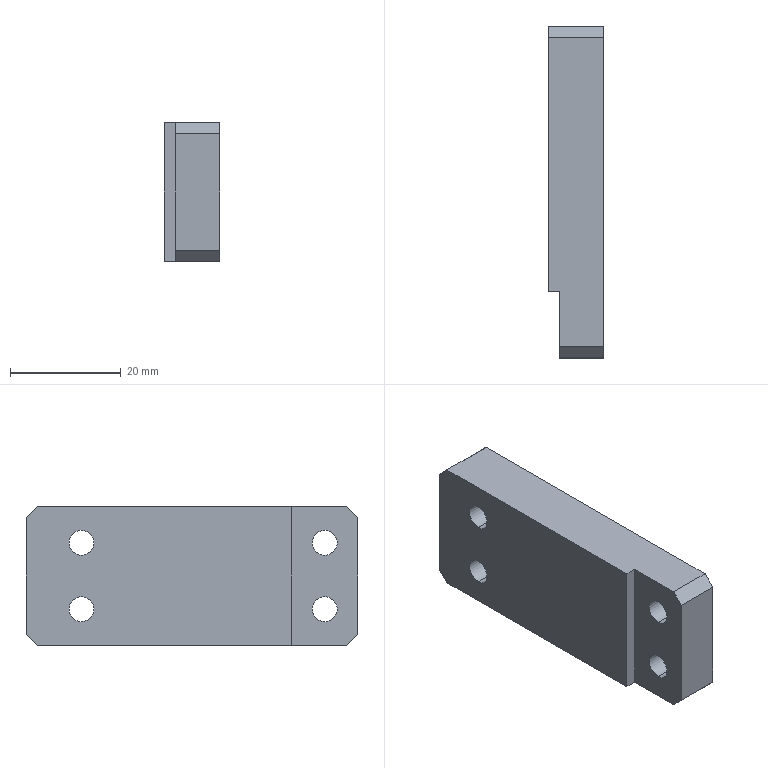Part | SolidWorks | features HoleWzd 2, Chamfer 1, Extrusion 1, ICE 1 | 1 solid | 32 faces | box 10 x 60 x 25 mm | volume 13123 mm3 | cylinder 16 | plane 16 | commonest cylinder face diameters 4.5 x8 8 x8
STEP:
#1=CARTESIAN_POINT('',(5.4,20.,10.));
#2=VERTEX_POINT('',#1);
#3=CARTESIAN_POINT('',(5.4,20.,2.));
#4=VERTEX_POINT('',#3);
#5=CARTESIAN_POINT('',(5.4,20.,6.));
#6=DIRECTION('',(1.,0.,0.));
#7=DIRECTION('',(0.,0.,-1.));
#8=AXIS2_PLACEMENT_3D('',#5,#6,#7);
#9=CIRCLE('',#8,4.);
#10=EDGE_CURVE('',#2,#4,#9,.T.);
#11=ORIENTED_EDGE('',*,*,#10,.F.);
#12=CARTESIAN_POINT('',(10.,20.,10.));
#13=VERTEX_POINT('',#12);
#14=CARTESIAN_POINT('',(10.,20.,10.));
#15=DIRECTION('',(1.,0.,0.));
#16=VECTOR('',#15,1000.);
#17=LINE('',#14,#16);
#18=EDGE_CURVE('',#2,#13,#17,.T.);
#19=ORIENTED_EDGE('',*,*,#18,.T.);
#20=CARTESIAN_POINT('',(10.,20.,2.));
#21=VERTEX_POINT('',#20);
#22=CARTESIAN_POINT('',(10.,20.,6.));
#23=DIRECTION('',(1.,0.,0.));
#24=DIRECTION('',(0.,0.,-1.));
#25=AXIS2_PLACEMENT_3D('',#22,#23,#24);
#26=CIRCLE('',#25,4.);
#27=EDGE_CURVE('',#13,#21,#26,.T.);
#28=ORIENTED_EDGE('',*,*,#27,.T.);
#29=CARTESIAN_POINT('',(10.,20.,2.));
#30=DIRECTION('',(1.,0.,0.));
#31=VECTOR('',#30,1000.);
#32=LINE('',#29,#31);
#33=EDGE_CURVE('',#4,#21,#32,.T.);
#34=ORIENTED_EDGE('',*,*,#33,.F.);
#35=EDGE_LOOP('',(#11,#19,#28,#34));
#36=FACE_OUTER_BOUND('',#35,.T.);
#37=CARTESIAN_POINT('',(10.,20.,6.));
#38=DIRECTION('',(1.,0.,0.));
#39=DIRECTION('',(0.,0.,-1.));
#40=AXIS2_PLACEMENT_3D('',#37,#38,#39);
#41=CYLINDRICAL_SURFACE('',#40,4.);
#42=ADVANCED_FACE('',(#36),#41,.F.);
#43=CARTESIAN_POINT('',(0.,20.,8.25));
#44=VERTEX_POINT('',#43);
#45=CARTESIAN_POINT('',(0.,20.,3.75));
#46=VERTEX_POINT('',#45);
#47=CARTESIAN_POINT('',(0.,20.,6.));
#48=DIRECTION('',(1.,0.,0.));
#49=DIRECTION('',(0.,0.,-1.));
#50=AXIS2_PLACEMENT_3D('',#47,#48,#49);
#51=CIRCLE('',#50,2.25);
#52=EDGE_CURVE('',#44,#46,#51,.T.);
#53=ORIENTED_EDGE('',*,*,#52,.F.);
#54=CARTESIAN_POINT('',(5.4,20.,8.25));
#55=VERTEX_POINT('',#54);
#56=CARTESIAN_POINT('',(10.,20.,8.25));
#57=DIRECTION('',(1.,0.,0.));
#58=VECTOR('',#57,1000.);
#59=LINE('',#56,#58);
#60=EDGE_CURVE('',#44,#55,#59,.T.);
#61=ORIENTED_EDGE('',*,*,#60,.T.);
#62=CARTESIAN_POINT('',(5.4,20.,3.75));
#63=VERTEX_POINT('',#62);
#64=CARTESIAN_POINT('',(5.4,20.,6.));
#65=DIRECTION('',(1.,0.,0.));
#66=DIRECTION('',(0.,0.,-1.));
#67=AXIS2_PLACEMENT_3D('',#64,#65,#66);
#68=CIRCLE('',#67,2.25);
#69=EDGE_CURVE('',#55,#63,#68,.T.);
#70=ORIENTED_EDGE('',*,*,#69,.T.);
#71=CARTESIAN_POINT('',(10.,20.,3.75));
#72=DIRECTION('',(1.,0.,0.));
#73=VECTOR('',#72,1000.);
#74=LINE('',#71,#73);
#75=EDGE_CURVE('',#46,#63,#74,.T.);
#76=ORIENTED_EDGE('',*,*,#75,.F.);
#77=EDGE_LOOP('',(#53,#61,#70,#76));
#78=FACE_OUTER_BOUND('',#77,.T.);
#79=CARTESIAN_POINT('',(10.,20.,6.));
#80=DIRECTION('',(1.,0.,0.));
#81=DIRECTION('',(0.,0.,-1.));
#82=AXIS2_PLACEMENT_3D('',#79,#80,#81);
#83=CYLINDRICAL_SURFACE('',#82,2.25);
#84=ADVANCED_FACE('',(#78),#83,.F.);
#85=CARTESIAN_POINT('',(5.4,20.,-2.));
#86=VERTEX_POINT('',#85);
#87=CARTESIAN_POINT('',(5.4,20.,-10.));
#88=VERTEX_POINT('',#87);
#89=CARTESIAN_POINT('',(5.4,20.,-6.));
#90=DIRECTION('',(1.,0.,0.));
#91=DIRECTION('',(0.,0.,-1.));
#92=AXIS2_PLACEMENT_3D('',#89,#90,#91);
#93=CIRCLE('',#92,4.);
#94=EDGE_CURVE('',#86,#88,#93,.T.);
#95=ORIENTED_EDGE('',*,*,#94,.F.);
#96=CARTESIAN_POINT('',(10.,20.,-2.));
#97=VERTEX_POINT('',#96);
#98=CARTESIAN_POINT('',(10.,20.,-2.));
#99=DIRECTION('',(1.,0.,0.));
#100=VECTOR('',#99,1000.);
#101=LINE('',#98,#100);
#102=EDGE_CURVE('',#86,#97,#101,.T.);
#103=ORIENTED_EDGE('',*,*,#102,.T.);
#104=CARTESIAN_POINT('',(10.,20.,-10.));
#105=VERTEX_POINT('',#104);
#106=CARTESIAN_POINT('',(10.,20.,-6.));
#107=DIRECTION('',(1.,0.,0.));
#108=DIRECTION('',(0.,0.,-1.));
#109=AXIS2_PLACEMENT_3D('',#106,#107,#108);
#110=CIRCLE('',#109,4.);
#111=EDGE_CURVE('',#97,#105,#110,.T.);
#112=ORIENTED_EDGE('',*,*,#111,.T.);
#113=CARTESIAN_POINT('',(10.,20.,-10.));
#114=DIRECTION('',(1.,0.,0.));
#115=VECTOR('',#114,1000.);
#116=LINE('',#113,#115);
#117=EDGE_CURVE('',#88,#105,#116,.T.);
#118=ORIENTED_EDGE('',*,*,#117,.F.);
#119=EDGE_LOOP('',(#95,#103,#112,#118));
#120=FACE_OUTER_BOUND('',#119,.T.);
#121=CARTESIAN_POINT('',(10.,20.,-6.));
#122=DIRECTION('',(1.,0.,0.));
#123=DIRECTION('',(0.,0.,-1.));
#124=AXIS2_PLACEMENT_3D('',#121,#122,#123);
#125=CYLINDRICAL_SURFACE('',#124,4.);
#126=ADVANCED_FACE('',(#120),#125,.F.);
#127=CARTESIAN_POINT('',(0.,20.,-3.75));
#128=VERTEX_POINT('',#127);
#129=CARTESIAN_POINT('',(0.,20.,-8.25));
#130=VERTEX_POINT('',#129);
#131=CARTESIAN_POINT('',(0.,20.,-6.));
#132=DIRECTION('',(1.,0.,0.));
#133=DIRECTION('',(0.,0.,-1.));
#134=AXIS2_PLACEMENT_3D('',#131,#132,#133);
#135=CIRCLE('',#134,2.25);
#136=EDGE_CURVE('',#128,#130,#135,.T.);
#137=ORIENTED_EDGE('',*,*,#136,.F.);
#138=CARTESIAN_POINT('',(5.4,20.,-3.75));
#139=VERTEX_POINT('',#138);
#140=CARTESIAN_POINT('',(10.,20.,-3.75));
#141=DIRECTION('',(1.,0.,0.));
#142=VECTOR('',#141,1000.);
#143=LINE('',#140,#142);
#144=EDGE_CURVE('',#128,#139,#143,.T.);
#145=ORIENTED_EDGE('',*,*,#144,.T.);
#146=CARTESIAN_POINT('',(5.4,20.,-8.25));
#147=VERTEX_POINT('',#146);
#148=CARTESIAN_POINT('',(5.4,20.,-6.));
#149=DIRECTION('',(1.,0.,0.));
#150=DIRECTION('',(0.,0.,-1.));
#151=AXIS2_PLACEMENT_3D('',#148,#149,#150);
#152=CIRCLE('',#151,2.25);
#153=EDGE_CURVE('',#139,#147,#152,.T.);
#154=ORIENTED_EDGE('',*,*,#153,.T.);
#155=CARTESIAN_POINT('',(10.,20.,-8.25));
#156=DIRECTION('',(1.,0.,0.));
#157=VECTOR('',#156,1000.);
#158=LINE('',#155,#157);
#159=EDGE_CURVE('',#130,#147,#158,.T.);
#160=ORIENTED_EDGE('',*,*,#159,.F.);
#161=EDGE_LOOP('',(#137,#145,#154,#160));
#162=FACE_OUTER_BOUND('',#161,.T.);
#163=CARTESIAN_POINT('',(10.,20.,-6.));
#164=DIRECTION('',(1.,0.,0.));
#165=DIRECTION('',(0.,0.,-1.));
#166=AXIS2_PLACEMENT_3D('',#163,#164,#165);
#167=CYLINDRICAL_SURFACE('',#166,2.25);
#168=ADVANCED_FACE('',(#162),#167,.F.);
#169=CARTESIAN_POINT('',(5.4,-24.,10.));
#170=VERTEX_POINT('',#169);
#171=CARTESIAN_POINT('',(5.4,-24.,2.));
#172=VERTEX_POINT('',#171);
#173=CARTESIAN_POINT('',(5.4,-24.,6.));
#174=DIRECTION('',(1.,0.,0.));
#175=DIRECTION('',(0.,0.,-1.));
#176=AXIS2_PLACEMENT_3D('',#173,#174,#175);
#177=CIRCLE('',#176,4.);
#178=EDGE_CURVE('',#170,#172,#177,.T.);
#179=ORIENTED_EDGE('',*,*,#178,.F.);
#180=CARTESIAN_POINT('',(10.,-24.,10.));
#181=VERTEX_POINT('',#180);
#182=CARTESIAN_POINT('',(10.,-24.,10.));
#183=DIRECTION('',(1.,0.,0.));
#184=VECTOR('',#183,1000.);
#185=LINE('',#182,#184);
#186=EDGE_CURVE('',#170,#181,#185,.T.);
#187=ORIENTED_EDGE('',*,*,#186,.T.);
#188=CARTESIAN_POINT('',(10.,-24.,2.));
#189=VERTEX_POINT('',#188);
#190=CARTESIAN_POINT('',(10.,-24.,6.));
#191=DIRECTION('',(1.,0.,0.));
#192=DIRECTION('',(0.,0.,-1.));
#193=AXIS2_PLACEMENT_3D('',#190,#191,#192);
#194=CIRCLE('',#193,4.);
#195=EDGE_CURVE('',#181,#189,#194,.T.);
#196=ORIENTED_EDGE('',*,*,#195,.T.);
#197=CARTESIAN_POINT('',(10.,-24.,2.));
#198=DIRECTION('',(1.,0.,0.));
#199=VECTOR('',#198,1000.);
#200=LINE('',#197,#199);
#201=EDGE_CURVE('',#172,#189,#200,.T.);
#202=ORIENTED_EDGE('',*,*,#201,.F.);
#203=EDGE_LOOP('',(#179,#187,#196,#202));
#204=FACE_OUTER_BOUND('',#203,.T.);
#205=CARTESIAN_POINT('',(10.,-24.,6.));
#206=DIRECTION('',(1.,0.,0.));
#207=DIRECTION('',(0.,0.,-1.));
#208=AXIS2_PLACEMENT_3D('',#205,#206,#207);
#209=CYLINDRICAL_SURFACE('',#208,4.);
#210=ADVANCED_FACE('',(#204),#209,.F.);
#211=CARTESIAN_POINT('',(2.,-24.,8.25));
#212=VERTEX_POINT('',#211);
#213=CARTESIAN_POINT('',(2.,-24.,3.75));
#214=VERTEX_POINT('',#213);
#215=CARTESIAN_POINT('',(2.,-24.,6.));
#216=DIRECTION('',(1.,0.,0.));
#217=DIRECTION('',(0.,0.,-1.));
#218=AXIS2_PLACEMENT_3D('',#215,#216,#217);
#219=CIRCLE('',#218,2.25);
#220=EDGE_CURVE('',#212,#214,#219,.T.);
#221=ORIENTED_EDGE('',*,*,#220,.F.);
#222=CARTESIAN_POINT('',(5.4,-24.,8.25));
#223=VERTEX_POINT('',#222);
#224=CARTESIAN_POINT('',(10.,-24.,8.25));
#225=DIRECTION('',(1.,0.,0.));
#226=VECTOR('',#225,1000.);
#227=LINE('',#224,#226);
#228=EDGE_CURVE('',#212,#223,#227,.T.);
#229=ORIENTED_EDGE('',*,*,#228,.T.);
#230=CARTESIAN_POINT('',(5.4,-24.,3.75));
#231=VERTEX_POINT('',#230);
#232=CARTESIAN_POINT('',(5.4,-24.,6.));
#233=DIRECTION('',(1.,0.,0.));
#234=DIRECTION('',(0.,0.,-1.));
#235=AXIS2_PLACEMENT_3D('',#232,#233,#234);
#236=CIRCLE('',#235,2.25);
#237=EDGE_CURVE('',#223,#231,#236,.T.);
#238=ORIENTED_EDGE('',*,*,#237,.T.);
#239=CARTESIAN_POINT('',(10.,-24.,3.75));
#240=DIRECTION('',(1.,0.,0.));
#241=VECTOR('',#240,1000.);
#242=LINE('',#239,#241);
#243=EDGE_CURVE('',#214,#231,#242,.T.);
#244=ORIENTED_EDGE('',*,*,#243,.F.);
#245=EDGE_LOOP('',(#221,#229,#238,#244));
#246=FACE_OUTER_BOUND('',#245,.T.);
#247=CARTESIAN_POINT('',(10.,-24.,6.));
#248=DIRECTION('',(1.,0.,0.));
#249=DIRECTION('',(0.,0.,-1.));
#250=AXIS2_PLACEMENT_3D('',#247,#248,#249);
#251=CYLINDRICAL_SURFACE('',#250,2.25);
#252=ADVANCED_FACE('',(#246),#251,.F.);
#253=CARTESIAN_POINT('',(5.4,-24.,-2.));
#254=VERTEX_POINT('',#253);
#255=CARTESIAN_POINT('',(5.4,-24.,-10.));
#256=VERTEX_POINT('',#255);
#257=CARTESIAN_POINT('',(5.4,-24.,-6.));
#258=DIRECTION('',(1.,0.,0.));
#259=DIRECTION('',(0.,0.,-1.));
#260=AXIS2_PLACEMENT_3D('',#257,#258,#259);
#261=CIRCLE('',#260,4.);
#262=EDGE_CURVE('',#254,#256,#261,.T.);
#263=ORIENTED_EDGE('',*,*,#262,.F.);
#264=CARTESIAN_POINT('',(10.,-24.,-2.));
#265=VERTEX_POINT('',#264);
#266=CARTESIAN_POINT('',(10.,-24.,-2.));
#267=DIRECTION('',(1.,0.,0.));
#268=VECTOR('',#267,1000.);
#269=LINE('',#266,#268);
#270=EDGE_CURVE('',#254,#265,#269,.T.);
#271=ORIENTED_EDGE('',*,*,#270,.T.);
#272=CARTESIAN_POINT('',(10.,-24.,-10.));
#273=VERTEX_POINT('',#272);
#274=CARTESIAN_POINT('',(10.,-24.,-6.));
#275=DIRECTION('',(1.,0.,0.));
#276=DIRECTION('',(0.,0.,-1.));
#277=AXIS2_PLACEMENT_3D('',#274,#275,#276);
#278=CIRCLE('',#277,4.);
#279=EDGE_CURVE('',#265,#273,#278,.T.);
#280=ORIENTED_EDGE('',*,*,#279,.T.);
#281=CARTESIAN_POINT('',(10.,-24.,-10.));
#282=DIRECTION('',(1.,0.,0.));
#283=VECTOR('',#282,1000.);
#284=LINE('',#281,#283);
#285=EDGE_CURVE('',#256,#273,#284,.T.);
#286=ORIENTED_EDGE('',*,*,#285,.F.);
#287=EDGE_LOOP('',(#263,#271,#280,#286));
#288=FACE_OUTER_BOUND('',#287,.T.);
#289=CARTESIAN_POINT('',(10.,-24.,-6.));
#290=DIRECTION('',(1.,0.,0.));
#291=DIRECTION('',(0.,0.,-1.));
#292=AXIS2_PLACEMENT_3D('',#289,#290,#291);
#293=CYLINDRICAL_SURFACE('',#292,4.);
#294=ADVANCED_FACE('',(#288),#293,.F.);
#295=CARTESIAN_POINT('',(2.,-24.,-3.75));
#296=VERTEX_POINT('',#295);
#297=CARTESIAN_POINT('',(2.,-24.,-8.25));
#298=VERTEX_POINT('',#297);
#299=CARTESIAN_POINT('',(2.,-24.,-6.));
#300=DIRECTION('',(1.,0.,0.));
#301=DIRECTION('',(0.,0.,-1.));
#302=AXIS2_PLACEMENT_3D('',#299,#300,#301);
#303=CIRCLE('',#302,2.25);
#304=EDGE_CURVE('',#296,#298,#303,.T.);
#305=ORIENTED_EDGE('',*,*,#304,.F.);
#306=CARTESIAN_POINT('',(5.4,-24.,-3.75));
#307=VERTEX_POINT('',#306);
#308=CARTESIAN_POINT('',(10.,-24.,-3.75));
#309=DIRECTION('',(1.,0.,0.));
#310=VECTOR('',#309,1000.);
#311=LINE('',#308,#310);
#312=EDGE_CURVE('',#296,#307,#311,.T.);
#313=ORIENTED_EDGE('',*,*,#312,.T.);
#314=CARTESIAN_POINT('',(5.4,-24.,-8.25));
#315=VERTEX_POINT('',#314);
#316=CARTESIAN_POINT('',(5.4,-24.,-6.));
#317=DIRECTION('',(1.,0.,0.));
#318=DIRECTION('',(0.,0.,-1.));
#319=AXIS2_PLACEMENT_3D('',#316,#317,#318);
#320=CIRCLE('',#319,2.25);
#321=EDGE_CURVE('',#307,#315,#320,.T.);
#322=ORIENTED_EDGE('',*,*,#321,.T.);
#323=CARTESIAN_POINT('',(10.,-24.,-8.25));
#324=DIRECTION('',(1.,0.,0.));
#325=VECTOR('',#324,1000.);
#326=LINE('',#323,#325);
#327=EDGE_CURVE('',#298,#315,#326,.T.);
#328=ORIENTED_EDGE('',*,*,#327,.F.);
#329=EDGE_LOOP('',(#305,#313,#322,#328));
#330=FACE_OUTER_BOUND('',#329,.T.);
#331=CARTESIAN_POINT('',(10.,-24.,-6.));
#332=DIRECTION('',(1.,0.,0.));
#333=DIRECTION('',(0.,0.,-1.));
#334=AXIS2_PLACEMENT_3D('',#331,#332,#333);
#335=CYLINDRICAL_SURFACE('',#334,2.25);
#336=ADVANCED_FACE('',(#330),#335,.F.);
#337=CARTESIAN_POINT('',(10.,20.,6.));
#338=DIRECTION('',(1.,0.,0.));
#339=DIRECTION('',(0.,0.,-1.));
#340=AXIS2_PLACEMENT_3D('',#337,#338,#339);
#341=CIRCLE('',#340,4.);
#342=EDGE_CURVE('',#21,#13,#341,.T.);
#343=ORIENTED_EDGE('',*,*,#342,.F.);
#344=ORIENTED_EDGE('',*,*,#27,.F.);
#345=EDGE_LOOP('',(#343,#344));
#346=FACE_BOUND('',#345,.T.);
#347=CARTESIAN_POINT('',(10.,20.,-6.));
#348=DIRECTION('',(1.,0.,0.));
#349=DIRECTION('',(0.,0.,-1.));
#350=AXIS2_PLACEMENT_3D('',#347,#348,#349);
#351=CIRCLE('',#350,4.);
#352=EDGE_CURVE('',#105,#97,#351,.T.);
#353=ORIENTED_EDGE('',*,*,#352,.F.);
#354=ORIENTED_EDGE('',*,*,#111,.F.);
#355=EDGE_LOOP('',(#353,#354));
#356=FACE_BOUND('',#355,.T.);
#357=CARTESIAN_POINT('',(10.,-24.,-6.));
#358=DIRECTION('',(1.,0.,0.));
#359=DIRECTION('',(0.,0.,-1.));
#360=AXIS2_PLACEMENT_3D('',#357,#358,#359);
#361=CIRCLE('',#360,4.);
#362=EDGE_CURVE('',#273,#265,#361,.T.);
#363=ORIENTED_EDGE('',*,*,#362,.F.);
#364=ORIENTED_EDGE('',*,*,#279,.F.);
#365=EDGE_LOOP('',(#363,#364));
#366=FACE_BOUND('',#365,.T.);
#367=CARTESIAN_POINT('',(10.,30.,-10.5));
#368=VERTEX_POINT('',#367);
#369=CARTESIAN_POINT('',(10.,30.,10.5));
#370=VERTEX_POINT('',#369);
#371=CARTESIAN_POINT('',(10.,30.,12.5));
#372=DIRECTION('',(0.,0.,1.));
#373=VECTOR('',#372,1000.);
#374=LINE('',#371,#373);
#375=EDGE_CURVE('',#368,#370,#374,.T.);
#376=ORIENTED_EDGE('',*,*,#375,.T.);
#377=CARTESIAN_POINT('',(10.,28.,12.5));
#378=VERTEX_POINT('',#377);
#379=CARTESIAN_POINT('',(10.,28.,12.5));
#380=DIRECTION('',(0.,-0.7071,0.7071));
#381=VECTOR('',#380,1000.);
#382=LINE('',#379,#381);
#383=EDGE_CURVE('',#370,#378,#382,.T.);
#384=ORIENTED_EDGE('',*,*,#383,.T.);
#385=CARTESIAN_POINT('',(10.,-28.,12.5));
#386=VERTEX_POINT('',#385);
#387=CARTESIAN_POINT('',(10.,-30.,12.5));
#388=DIRECTION('',(0.,-1.,0.));
#389=VECTOR('',#388,1000.);
#390=LINE('',#387,#389);
#391=EDGE_CURVE('',#378,#386,#390,.T.);
#392=ORIENTED_EDGE('',*,*,#391,.T.);
#393=CARTESIAN_POINT('',(10.,-30.,10.5));
#394=VERTEX_POINT('',#393);
#395=CARTESIAN_POINT('',(10.,-30.,10.5));
#396=DIRECTION('',(0.,-0.7071,-0.7071));
#397=VECTOR('',#396,1000.);
#398=LINE('',#395,#397);
#399=EDGE_CURVE('',#386,#394,#398,.T.);
#400=ORIENTED_EDGE('',*,*,#399,.T.);
#401=CARTESIAN_POINT('',(10.,-30.,-10.5));
#402=VERTEX_POINT('',#401);
#403=CARTESIAN_POINT('',(10.,-30.,12.5));
#404=DIRECTION('',(0.,0.,-1.));
#405=VECTOR('',#404,1000.);
#406=LINE('',#403,#405);
#407=EDGE_CURVE('',#394,#402,#406,.T.);
#408=ORIENTED_EDGE('',*,*,#407,.T.);
#409=CARTESIAN_POINT('',(10.,-28.,-12.5));
#410=VERTEX_POINT('',#409);
#411=CARTESIAN_POINT('',(10.,-28.,-12.5));
#412=DIRECTION('',(0.,0.7071,-0.7071));
#413=VECTOR('',#412,1000.);
#414=LINE('',#411,#413);
#415=EDGE_CURVE('',#402,#410,#414,.T.);
#416=ORIENTED_EDGE('',*,*,#415,.T.);
#417=CARTESIAN_POINT('',(10.,28.,-12.5));
#418=VERTEX_POINT('',#417);
#419=CARTESIAN_POINT('',(10.,-30.,-12.5));
#420=DIRECTION('',(0.,1.,0.));
#421=VECTOR('',#420,1000.);
#422=LINE('',#419,#421);
#423=EDGE_CURVE('',#410,#418,#422,.T.);
#424=ORIENTED_EDGE('',*,*,#423,.T.);
#425=CARTESIAN_POINT('',(10.,30.,-10.5));
#426=DIRECTION('',(0.,0.7071,0.7071));
#427=VECTOR('',#426,1000.);
#428=LINE('',#425,#427);
#429=EDGE_CURVE('',#418,#368,#428,.T.);
#430=ORIENTED_EDGE('',*,*,#429,.T.);
#431=EDGE_LOOP('',(#376,#384,#392,#400,#408,#416,#424,#430));
#432=FACE_OUTER_BOUND('',#431,.T.);
#433=CARTESIAN_POINT('',(10.,-24.,6.));
#434=DIRECTION('',(1.,0.,0.));
#435=DIRECTION('',(0.,0.,-1.));
#436=AXIS2_PLACEMENT_3D('',#433,#434,#435);
#437=CIRCLE('',#436,4.);
#438=EDGE_CURVE('',#189,#181,#437,.T.);
#439=ORIENTED_EDGE('',*,*,#438,.F.);
#440=ORIENTED_EDGE('',*,*,#195,.F.);
#441=EDGE_LOOP('',(#439,#440));
#442=FACE_BOUND('',#441,.T.);
#443=CARTESIAN_POINT('',(10.,0.,0.));
#444=DIRECTION('',(-1.,0.,0.));
#445=DIRECTION('',(0.,0.,1.));
#446=AXIS2_PLACEMENT_3D('',#443,#444,#445);
#447=PLANE('',#446);
#448=ADVANCED_FACE('',(#346,#356,#366,#432,#442),#447,.F.);
#449=CARTESIAN_POINT('',(0.,-18.,-12.5));
#450=VERTEX_POINT('',#449);
#451=CARTESIAN_POINT('',(0.,28.,-12.5));
#452=VERTEX_POINT('',#451);
#453=CARTESIAN_POINT('',(0.,-30.,-12.5));
#454=DIRECTION('',(0.,1.,0.));
#455=VECTOR('',#454,1000.);
#456=LINE('',#453,#455);
#457=EDGE_CURVE('',#450,#452,#456,.T.);
#458=ORIENTED_EDGE('',*,*,#457,.T.);
#459=CARTESIAN_POINT('',(10.,28.,-12.5));
#460=DIRECTION('',(1.,0.,0.));
#461=VECTOR('',#460,1000.);
#462=LINE('',#459,#461);
#463=EDGE_CURVE('',#452,#418,#462,.T.);
#464=ORIENTED_EDGE('',*,*,#463,.T.);
#465=ORIENTED_EDGE('',*,*,#423,.F.);
#466=CARTESIAN_POINT('',(2.,-28.,-12.5));
#467=VERTEX_POINT('',#466);
#468=CARTESIAN_POINT('',(10.,-28.,-12.5));
#469=DIRECTION('',(-1.,0.,0.));
#470=VECTOR('',#469,1000.);
#471=LINE('',#468,#470);
#472=EDGE_CURVE('',#410,#467,#471,.T.);
#473=ORIENTED_EDGE('',*,*,#472,.T.);
#474=CARTESIAN_POINT('',(2.,-18.,-12.5));
#475=VERTEX_POINT('',#474);
#476=CARTESIAN_POINT('',(2.,-30.,-12.5));
#477=DIRECTION('',(0.,-1.,0.));
#478=VECTOR('',#477,1000.);
#479=LINE('',#476,#478);
#480=EDGE_CURVE('',#475,#467,#479,.T.);
#481=ORIENTED_EDGE('',*,*,#480,.F.);
#482=CARTESIAN_POINT('',(2.,-18.,-12.5));
#483=DIRECTION('',(-1.,0.,0.));
#484=VECTOR('',#483,1000.);
#485=LINE('',#482,#484);
#486=EDGE_CURVE('',#475,#450,#485,.T.);
#487=ORIENTED_EDGE('',*,*,#486,.T.);
#488=EDGE_LOOP('',(#458,#464,#465,#473,#481,#487));
#489=FACE_OUTER_BOUND('',#488,.T.);
#490=CARTESIAN_POINT('',(10.,-30.,-12.5));
#491=DIRECTION('',(0.,0.,1.));
#492=DIRECTION('',(1.,0.,0.));
#493=AXIS2_PLACEMENT_3D('',#490,#491,#492);
#494=PLANE('',#493);
#495=ADVANCED_FACE('',(#489),#494,.F.);
#496=CARTESIAN_POINT('',(0.,30.,-10.5));
#497=VERTEX_POINT('',#496);
#498=CARTESIAN_POINT('',(0.,30.,10.5));
#499=VERTEX_POINT('',#498);
#500=CARTESIAN_POINT('',(0.,30.,12.5));
#501=DIRECTION('',(0.,0.,1.));
#502=VECTOR('',#501,1000.);
#503=LINE('',#500,#502);
#504=EDGE_CURVE('',#497,#499,#503,.T.);
#505=ORIENTED_EDGE('',*,*,#504,.T.);
#506=CARTESIAN_POINT('',(10.,30.,10.5));
#507=DIRECTION('',(1.,0.,0.));
#508=VECTOR('',#507,1000.);
#509=LINE('',#506,#508);
#510=EDGE_CURVE('',#499,#370,#509,.T.);
#511=ORIENTED_EDGE('',*,*,#510,.T.);
#512=ORIENTED_EDGE('',*,*,#375,.F.);
#513=CARTESIAN_POINT('',(10.,30.,-10.5));
#514=DIRECTION('',(-1.,0.,0.));
#515=VECTOR('',#514,1000.);
#516=LINE('',#513,#515);
#517=EDGE_CURVE('',#368,#497,#516,.T.);
#518=ORIENTED_EDGE('',*,*,#517,.T.);
#519=EDGE_LOOP('',(#505,#511,#512,#518));
#520=FACE_OUTER_BOUND('',#519,.T.);
#521=CARTESIAN_POINT('',(10.,30.,12.5));
#522=DIRECTION('',(0.,-1.,0.));
#523=DIRECTION('',(0.,0.,-1.));
#524=AXIS2_PLACEMENT_3D('',#521,#522,#523);
#525=PLANE('',#524);
#526=ADVANCED_FACE('',(#520),#525,.F.);
#527=ORIENTED_EDGE('',*,*,#391,.F.);
#528=CARTESIAN_POINT('',(0.,28.,12.5));
#529=VERTEX_POINT('',#528);
#530=CARTESIAN_POINT('',(10.,28.,12.5));
#531=DIRECTION('',(-1.,0.,0.));
#532=VECTOR('',#531,1000.);
#533=LINE('',#530,#532);
#534=EDGE_CURVE('',#378,#529,#533,.T.);
#535=ORIENTED_EDGE('',*,*,#534,.T.);
#536=CARTESIAN_POINT('',(0.,-18.,12.5));
#537=VERTEX_POINT('',#536);
#538=CARTESIAN_POINT('',(0.,-30.,12.5));
#539=DIRECTION('',(0.,-1.,0.));
#540=VECTOR('',#539,1000.);
#541=LINE('',#538,#540);
#542=EDGE_CURVE('',#529,#537,#541,.T.);
#543=ORIENTED_EDGE('',*,*,#542,.T.);
#544=CARTESIAN_POINT('',(2.,-18.,12.5));
#545=VERTEX_POINT('',#544);
#546=CARTESIAN_POINT('',(2.,-18.,12.5));
#547=DIRECTION('',(-1.,0.,0.));
#548=VECTOR('',#547,1000.);
#549=LINE('',#546,#548);
#550=EDGE_CURVE('',#545,#537,#549,.T.);
#551=ORIENTED_EDGE('',*,*,#550,.F.);
#552=CARTESIAN_POINT('',(2.,-28.,12.5));
#553=VERTEX_POINT('',#552);
#554=CARTESIAN_POINT('',(2.,-30.,12.5));
#555=DIRECTION('',(0.,1.,0.));
#556=VECTOR('',#555,1000.);
#557=LINE('',#554,#556);
#558=EDGE_CURVE('',#553,#545,#557,.T.);
#559=ORIENTED_EDGE('',*,*,#558,.F.);
#560=CARTESIAN_POINT('',(10.,-28.,12.5));
#561=DIRECTION('',(1.,0.,0.));
#562=VECTOR('',#561,1000.);
#563=LINE('',#560,#562);
#564=EDGE_CURVE('',#553,#386,#563,.T.);
#565=ORIENTED_EDGE('',*,*,#564,.T.);
#566=EDGE_LOOP('',(#527,#535,#543,#551,#559,#565));
#567=FACE_OUTER_BOUND('',#566,.T.);
#568=CARTESIAN_POINT('',(10.,-30.,12.5));
#569=DIRECTION('',(0.,0.,-1.));
#570=DIRECTION('',(-1.,0.,0.));
#571=AXIS2_PLACEMENT_3D('',#568,#569,#570);
#572=PLANE('',#571);
#573=ADVANCED_FACE('',(#567),#572,.F.);
#574=ORIENTED_EDGE('',*,*,#407,.F.);
#575=CARTESIAN_POINT('',(2.,-30.,10.5));
#576=VERTEX_POINT('',#575);
#577=CARTESIAN_POINT('',(10.,-30.,10.5));
#578=DIRECTION('',(-1.,0.,0.));
#579=VECTOR('',#578,1000.);
#580=LINE('',#577,#579);
#581=EDGE_CURVE('',#394,#576,#580,.T.);
#582=ORIENTED_EDGE('',*,*,#581,.T.);
#583=CARTESIAN_POINT('',(2.,-30.,-10.5));
#584=VERTEX_POINT('',#583);
#585=CARTESIAN_POINT('',(2.,-30.,-12.5));
#586=DIRECTION('',(0.,0.,1.));
#587=VECTOR('',#586,1000.);
#588=LINE('',#585,#587);
#589=EDGE_CURVE('',#584,#576,#588,.T.);
#590=ORIENTED_EDGE('',*,*,#589,.F.);
#591=CARTESIAN_POINT('',(10.,-30.,-10.5));
#592=DIRECTION('',(1.,0.,0.));
#593=VECTOR('',#592,1000.);
#594=LINE('',#591,#593);
#595=EDGE_CURVE('',#584,#402,#594,.T.);
#596=ORIENTED_EDGE('',*,*,#595,.T.);
#597=EDGE_LOOP('',(#574,#582,#590,#596));
#598=FACE_OUTER_BOUND('',#597,.T.);
#599=CARTESIAN_POINT('',(10.,-30.,12.5));
#600=DIRECTION('',(0.,1.,0.));
#601=DIRECTION('',(0.,0.,1.));
#602=AXIS2_PLACEMENT_3D('',#599,#600,#601);
#603=PLANE('',#602);
#604=ADVANCED_FACE('',(#598),#603,.F.);
#605=CARTESIAN_POINT('',(0.,20.,6.));
#606=DIRECTION('',(1.,0.,0.));
#607=DIRECTION('',(0.,0.,-1.));
#608=AXIS2_PLACEMENT_3D('',#605,#606,#607);
#609=CIRCLE('',#608,2.25);
#610=EDGE_CURVE('',#46,#44,#609,.T.);
#611=ORIENTED_EDGE('',*,*,#610,.T.);
#612=ORIENTED_EDGE('',*,*,#52,.T.);
#613=EDGE_LOOP('',(#611,#612));
#614=FACE_BOUND('',#613,.T.);
#615=CARTESIAN_POINT('',(0.,20.,-6.));
#616=DIRECTION('',(1.,0.,0.));
#617=DIRECTION('',(0.,0.,-1.));
#618=AXIS2_PLACEMENT_3D('',#615,#616,#617);
#619=CIRCLE('',#618,2.25);
#620=EDGE_CURVE('',#130,#128,#619,.T.);
#621=ORIENTED_EDGE('',*,*,#620,.T.);
#622=ORIENTED_EDGE('',*,*,#136,.T.);
#623=EDGE_LOOP('',(#621,#622));
#624=FACE_BOUND('',#623,.T.);
#625=ORIENTED_EDGE('',*,*,#542,.F.);
#626=CARTESIAN_POINT('',(0.,20.25,20.25));
#627=DIRECTION('',(0.,0.7071,-0.7071));
#628=VECTOR('',#627,1000.);
#629=LINE('',#626,#628);
#630=EDGE_CURVE('',#529,#499,#629,.T.);
#631=ORIENTED_EDGE('',*,*,#630,.T.);
#632=ORIENTED_EDGE('',*,*,#504,.F.);
#633=CARTESIAN_POINT('',(0.,20.25,-20.25));
#634=DIRECTION('',(0.,-0.7071,-0.7071));
#635=VECTOR('',#634,1000.);
#636=LINE('',#633,#635);
#637=EDGE_CURVE('',#497,#452,#636,.T.);
#638=ORIENTED_EDGE('',*,*,#637,.T.);
#639=ORIENTED_EDGE('',*,*,#457,.F.);
#640=CARTESIAN_POINT('',(0.,-18.,-12.5));
#641=DIRECTION('',(0.,0.,-1.));
#642=VECTOR('',#641,1000.);
#643=LINE('',#640,#642);
#644=EDGE_CURVE('',#537,#450,#643,.T.);
#645=ORIENTED_EDGE('',*,*,#644,.F.);
#646=EDGE_LOOP('',(#625,#631,#632,#638,#639,#645));
#647=FACE_OUTER_BOUND('',#646,.T.);
#648=CARTESIAN_POINT('',(0.,0.,0.));
#649=DIRECTION('',(-1.,0.,0.));
#650=DIRECTION('',(0.,0.,1.));
#651=AXIS2_PLACEMENT_3D('',#648,#649,#650);
#652=PLANE('',#651);
#653=ADVANCED_FACE('',(#614,#624,#647),#652,.T.);
#654=ORIENTED_EDGE('',*,*,#644,.T.);
#655=ORIENTED_EDGE('',*,*,#486,.F.);
#656=CARTESIAN_POINT('',(2.,-18.,-12.5));
#657=DIRECTION('',(0.,0.,-1.));
#658=VECTOR('',#657,1000.);
#659=LINE('',#656,#658);
#660=EDGE_CURVE('',#545,#475,#659,.T.);
#661=ORIENTED_EDGE('',*,*,#660,.F.);
#662=ORIENTED_EDGE('',*,*,#550,.T.);
#663=EDGE_LOOP('',(#654,#655,#661,#662));
#664=FACE_OUTER_BOUND('',#663,.T.);
#665=CARTESIAN_POINT('',(2.,-18.,-12.5));
#666=DIRECTION('',(0.,1.,0.));
#667=DIRECTION('',(0.,0.,1.));
#668=AXIS2_PLACEMENT_3D('',#665,#666,#667);
#669=PLANE('',#668);
#670=ADVANCED_FACE('',(#664),#669,.F.);
#671=CARTESIAN_POINT('',(2.,-24.,6.));
#672=DIRECTION('',(1.,0.,0.));
#673=DIRECTION('',(0.,0.,-1.));
#674=AXIS2_PLACEMENT_3D('',#671,#672,#673);
#675=CIRCLE('',#674,2.25);
#676=EDGE_CURVE('',#214,#212,#675,.T.);
#677=ORIENTED_EDGE('',*,*,#676,.T.);
#678=ORIENTED_EDGE('',*,*,#220,.T.);
#679=EDGE_LOOP('',(#677,#678));
#680=FACE_BOUND('',#679,.T.);
#681=CARTESIAN_POINT('',(2.,-24.,-6.));
#682=DIRECTION('',(1.,0.,0.));
#683=DIRECTION('',(0.,0.,-1.));
#684=AXIS2_PLACEMENT_3D('',#681,#682,#683);
#685=CIRCLE('',#684,2.25);
#686=EDGE_CURVE('',#298,#296,#685,.T.);
#687=ORIENTED_EDGE('',*,*,#686,.T.);
#688=ORIENTED_EDGE('',*,*,#304,.T.);
#689=EDGE_LOOP('',(#687,#688));
#690=FACE_BOUND('',#689,.T.);
#691=ORIENTED_EDGE('',*,*,#589,.T.);
#692=CARTESIAN_POINT('',(2.,-30.,10.5));
#693=DIRECTION('',(0.,0.7071,0.7071));
#694=VECTOR('',#693,1000.);
#695=LINE('',#692,#694);
#696=EDGE_CURVE('',#576,#553,#695,.T.);
#697=ORIENTED_EDGE('',*,*,#696,.T.);
#698=ORIENTED_EDGE('',*,*,#558,.T.);
#699=ORIENTED_EDGE('',*,*,#660,.T.);
#700=ORIENTED_EDGE('',*,*,#480,.T.);
#701=CARTESIAN_POINT('',(2.,-28.,-12.5));
#702=DIRECTION('',(0.,-0.7071,0.7071));
#703=VECTOR('',#702,1000.);
#704=LINE('',#701,#703);
#705=EDGE_CURVE('',#467,#584,#704,.T.);
#706=ORIENTED_EDGE('',*,*,#705,.T.);
#707=EDGE_LOOP('',(#691,#697,#698,#699,#700,#706));
#708=FACE_OUTER_BOUND('',#707,.T.);
#709=CARTESIAN_POINT('',(2.,0.,0.));
#710=DIRECTION('',(1.,0.,0.));
#711=DIRECTION('',(0.,0.,-1.));
#712=AXIS2_PLACEMENT_3D('',#709,#710,#711);
#713=PLANE('',#712);
#714=ADVANCED_FACE('',(#680,#690,#708),#713,.F.);
#715=ORIENTED_EDGE('',*,*,#312,.F.);
#716=ORIENTED_EDGE('',*,*,#686,.F.);
#717=ORIENTED_EDGE('',*,*,#327,.T.);
#718=CARTESIAN_POINT('',(5.4,-24.,-6.));
#719=DIRECTION('',(1.,0.,0.));
#720=DIRECTION('',(0.,0.,-1.));
#721=AXIS2_PLACEMENT_3D('',#718,#719,#720);
#722=CIRCLE('',#721,2.25);
#723=EDGE_CURVE('',#315,#307,#722,.T.);
#724=ORIENTED_EDGE('',*,*,#723,.T.);
#725=EDGE_LOOP('',(#715,#716,#717,#724));
#726=FACE_OUTER_BOUND('',#725,.T.);
#727=CARTESIAN_POINT('',(10.,-24.,-6.));
#728=DIRECTION('',(1.,0.,0.));
#729=DIRECTION('',(0.,0.,-1.));
#730=AXIS2_PLACEMENT_3D('',#727,#728,#729);
#731=CYLINDRICAL_SURFACE('',#730,2.25);
#732=ADVANCED_FACE('',(#726),#731,.F.);
#733=ORIENTED_EDGE('',*,*,#723,.F.);
#734=ORIENTED_EDGE('',*,*,#321,.F.);
#735=EDGE_LOOP('',(#733,#734));
#736=FACE_BOUND('',#735,.T.);
#737=CARTESIAN_POINT('',(5.4,-24.,-6.));
#738=DIRECTION('',(1.,0.,0.));
#739=DIRECTION('',(0.,0.,-1.));
#740=AXIS2_PLACEMENT_3D('',#737,#738,#739);
#741=CIRCLE('',#740,4.);
#742=EDGE_CURVE('',#256,#254,#741,.T.);
#743=ORIENTED_EDGE('',*,*,#742,.T.);
#744=ORIENTED_EDGE('',*,*,#262,.T.);
#745=EDGE_LOOP('',(#743,#744));
#746=FACE_OUTER_BOUND('',#745,.T.);
#747=CARTESIAN_POINT('',(5.4,-21.75,-6.));
#748=DIRECTION('',(-1.,0.,0.));
#749=DIRECTION('',(0.,0.,1.));
#750=AXIS2_PLACEMENT_3D('',#747,#748,#749);
#751=PLANE('',#750);
#752=ADVANCED_FACE('',(#736,#746),#751,.F.);
#753=ORIENTED_EDGE('',*,*,#270,.F.);
#754=ORIENTED_EDGE('',*,*,#742,.F.);
#755=ORIENTED_EDGE('',*,*,#285,.T.);
#756=ORIENTED_EDGE('',*,*,#362,.T.);
#757=EDGE_LOOP('',(#753,#754,#755,#756));
#758=FACE_OUTER_BOUND('',#757,.T.);
#759=CARTESIAN_POINT('',(10.,-24.,-6.));
#760=DIRECTION('',(1.,0.,0.));
#761=DIRECTION('',(0.,0.,-1.));
#762=AXIS2_PLACEMENT_3D('',#759,#760,#761);
#763=CYLINDRICAL_SURFACE('',#762,4.);
#764=ADVANCED_FACE('',(#758),#763,.F.);
#765=ORIENTED_EDGE('',*,*,#228,.F.);
#766=ORIENTED_EDGE('',*,*,#676,.F.);
#767=ORIENTED_EDGE('',*,*,#243,.T.);
#768=CARTESIAN_POINT('',(5.4,-24.,6.));
#769=DIRECTION('',(1.,0.,0.));
#770=DIRECTION('',(0.,0.,-1.));
#771=AXIS2_PLACEMENT_3D('',#768,#769,#770);
#772=CIRCLE('',#771,2.25);
#773=EDGE_CURVE('',#231,#223,#772,.T.);
#774=ORIENTED_EDGE('',*,*,#773,.T.);
#775=EDGE_LOOP('',(#765,#766,#767,#774));
#776=FACE_OUTER_BOUND('',#775,.T.);
#777=CARTESIAN_POINT('',(10.,-24.,6.));
#778=DIRECTION('',(1.,0.,0.));
#779=DIRECTION('',(0.,0.,-1.));
#780=AXIS2_PLACEMENT_3D('',#777,#778,#779);
#781=CYLINDRICAL_SURFACE('',#780,2.25);
#782=ADVANCED_FACE('',(#776),#781,.F.);
#783=ORIENTED_EDGE('',*,*,#773,.F.);
#784=ORIENTED_EDGE('',*,*,#237,.F.);
#785=EDGE_LOOP('',(#783,#784));
#786=FACE_BOUND('',#785,.T.);
#787=CARTESIAN_POINT('',(5.4,-24.,6.));
#788=DIRECTION('',(1.,0.,0.));
#789=DIRECTION('',(0.,0.,-1.));
#790=AXIS2_PLACEMENT_3D('',#787,#788,#789);
#791=CIRCLE('',#790,4.);
#792=EDGE_CURVE('',#172,#170,#791,.T.);
#793=ORIENTED_EDGE('',*,*,#792,.T.);
#794=ORIENTED_EDGE('',*,*,#178,.T.);
#795=EDGE_LOOP('',(#793,#794));
#796=FACE_OUTER_BOUND('',#795,.T.);
#797=CARTESIAN_POINT('',(5.4,-21.75,6.));
#798=DIRECTION('',(-1.,0.,0.));
#799=DIRECTION('',(0.,0.,1.));
#800=AXIS2_PLACEMENT_3D('',#797,#798,#799);
#801=PLANE('',#800);
#802=ADVANCED_FACE('',(#786,#796),#801,.F.);
#803=ORIENTED_EDGE('',*,*,#186,.F.);
#804=ORIENTED_EDGE('',*,*,#792,.F.);
#805=ORIENTED_EDGE('',*,*,#201,.T.);
#806=ORIENTED_EDGE('',*,*,#438,.T.);
#807=EDGE_LOOP('',(#803,#804,#805,#806));
#808=FACE_OUTER_BOUND('',#807,.T.);
#809=CARTESIAN_POINT('',(10.,-24.,6.));
#810=DIRECTION('',(1.,0.,0.));
#811=DIRECTION('',(0.,0.,-1.));
#812=AXIS2_PLACEMENT_3D('',#809,#810,#811);
#813=CYLINDRICAL_SURFACE('',#812,4.);
#814=ADVANCED_FACE('',(#808),#813,.F.);
#815=ORIENTED_EDGE('',*,*,#144,.F.);
#816=ORIENTED_EDGE('',*,*,#620,.F.);
#817=ORIENTED_EDGE('',*,*,#159,.T.);
#818=CARTESIAN_POINT('',(5.4,20.,-6.));
#819=DIRECTION('',(1.,0.,0.));
#820=DIRECTION('',(0.,0.,-1.));
#821=AXIS2_PLACEMENT_3D('',#818,#819,#820);
#822=CIRCLE('',#821,2.25);
#823=EDGE_CURVE('',#147,#139,#822,.T.);
#824=ORIENTED_EDGE('',*,*,#823,.T.);
#825=EDGE_LOOP('',(#815,#816,#817,#824));
#826=FACE_OUTER_BOUND('',#825,.T.);
#827=CARTESIAN_POINT('',(10.,20.,-6.));
#828=DIRECTION('',(1.,0.,0.));
#829=DIRECTION('',(0.,0.,-1.));
#830=AXIS2_PLACEMENT_3D('',#827,#828,#829);
#831=CYLINDRICAL_SURFACE('',#830,2.25);
#832=ADVANCED_FACE('',(#826),#831,.F.);
#833=ORIENTED_EDGE('',*,*,#823,.F.);
#834=ORIENTED_EDGE('',*,*,#153,.F.);
#835=EDGE_LOOP('',(#833,#834));
#836=FACE_BOUND('',#835,.T.);
#837=CARTESIAN_POINT('',(5.4,20.,-6.));
#838=DIRECTION('',(1.,0.,0.));
#839=DIRECTION('',(0.,0.,-1.));
#840=AXIS2_PLACEMENT_3D('',#837,#838,#839);
#841=CIRCLE('',#840,4.);
#842=EDGE_CURVE('',#88,#86,#841,.T.);
#843=ORIENTED_EDGE('',*,*,#842,.T.);
#844=ORIENTED_EDGE('',*,*,#94,.T.);
#845=EDGE_LOOP('',(#843,#844));
#846=FACE_OUTER_BOUND('',#845,.T.);
#847=CARTESIAN_POINT('',(5.4,22.25,-6.));
#848=DIRECTION('',(-1.,0.,0.));
#849=DIRECTION('',(0.,0.,1.));
#850=AXIS2_PLACEMENT_3D('',#847,#848,#849);
#851=PLANE('',#850);
#852=ADVANCED_FACE('',(#836,#846),#851,.F.);
#853=ORIENTED_EDGE('',*,*,#102,.F.);
#854=ORIENTED_EDGE('',*,*,#842,.F.);
#855=ORIENTED_EDGE('',*,*,#117,.T.);
#856=ORIENTED_EDGE('',*,*,#352,.T.);
#857=EDGE_LOOP('',(#853,#854,#855,#856));
#858=FACE_OUTER_BOUND('',#857,.T.);
#859=CARTESIAN_POINT('',(10.,20.,-6.));
#860=DIRECTION('',(1.,0.,0.));
#861=DIRECTION('',(0.,0.,-1.));
#862=AXIS2_PLACEMENT_3D('',#859,#860,#861);
#863=CYLINDRICAL_SURFACE('',#862,4.);
#864=ADVANCED_FACE('',(#858),#863,.F.);
#865=ORIENTED_EDGE('',*,*,#60,.F.);
#866=ORIENTED_EDGE('',*,*,#610,.F.);
#867=ORIENTED_EDGE('',*,*,#75,.T.);
#868=CARTESIAN_POINT('',(5.4,20.,6.));
#869=DIRECTION('',(1.,0.,0.));
#870=DIRECTION('',(0.,0.,-1.));
#871=AXIS2_PLACEMENT_3D('',#868,#869,#870);
#872=CIRCLE('',#871,2.25);
#873=EDGE_CURVE('',#63,#55,#872,.T.);
#874=ORIENTED_EDGE('',*,*,#873,.T.);
#875=EDGE_LOOP('',(#865,#866,#867,#874));
#876=FACE_OUTER_BOUND('',#875,.T.);
#877=CARTESIAN_POINT('',(10.,20.,6.));
#878=DIRECTION('',(1.,0.,0.));
#879=DIRECTION('',(0.,0.,-1.));
#880=AXIS2_PLACEMENT_3D('',#877,#878,#879);
#881=CYLINDRICAL_SURFACE('',#880,2.25);
#882=ADVANCED_FACE('',(#876),#881,.F.);
#883=ORIENTED_EDGE('',*,*,#873,.F.);
#884=ORIENTED_EDGE('',*,*,#69,.F.);
#885=EDGE_LOOP('',(#883,#884));
#886=FACE_BOUND('',#885,.T.);
#887=CARTESIAN_POINT('',(5.4,20.,6.));
#888=DIRECTION('',(1.,0.,0.));
#889=DIRECTION('',(0.,0.,-1.));
#890=AXIS2_PLACEMENT_3D('',#887,#888,#889);
#891=CIRCLE('',#890,4.);
#892=EDGE_CURVE('',#4,#2,#891,.T.);
#893=ORIENTED_EDGE('',*,*,#892,.T.);
#894=ORIENTED_EDGE('',*,*,#10,.T.);
#895=EDGE_LOOP('',(#893,#894));
#896=FACE_OUTER_BOUND('',#895,.T.);
#897=CARTESIAN_POINT('',(5.4,22.25,6.));
#898=DIRECTION('',(-1.,0.,0.));
#899=DIRECTION('',(0.,0.,1.));
#900=AXIS2_PLACEMENT_3D('',#897,#898,#899);
#901=PLANE('',#900);
#902=ADVANCED_FACE('',(#886,#896),#901,.F.);
#903=ORIENTED_EDGE('',*,*,#18,.F.);
#904=ORIENTED_EDGE('',*,*,#892,.F.);
#905=ORIENTED_EDGE('',*,*,#33,.T.);
#906=ORIENTED_EDGE('',*,*,#342,.T.);
#907=EDGE_LOOP('',(#903,#904,#905,#906));
#908=FACE_OUTER_BOUND('',#907,.T.);
#909=CARTESIAN_POINT('',(10.,20.,6.));
#910=DIRECTION('',(1.,0.,0.));
#911=DIRECTION('',(0.,0.,-1.));
#912=AXIS2_PLACEMENT_3D('',#909,#910,#911);
#913=CYLINDRICAL_SURFACE('',#912,4.);
#914=ADVANCED_FACE('',(#908),#913,.F.);
#915=ORIENTED_EDGE('',*,*,#383,.F.);
#916=ORIENTED_EDGE('',*,*,#510,.F.);
#917=ORIENTED_EDGE('',*,*,#630,.F.);
#918=ORIENTED_EDGE('',*,*,#534,.F.);
#919=EDGE_LOOP('',(#915,#916,#917,#918));
#920=FACE_OUTER_BOUND('',#919,.T.);
#921=CARTESIAN_POINT('',(10.,28.,12.5));
#922=DIRECTION('',(0.,-0.7071,-0.7071));
#923=DIRECTION('',(-1.,0.,0.));
#924=AXIS2_PLACEMENT_3D('',#921,#922,#923);
#925=PLANE('',#924);
#926=ADVANCED_FACE('',(#920),#925,.F.);
#927=ORIENTED_EDGE('',*,*,#429,.F.);
#928=ORIENTED_EDGE('',*,*,#463,.F.);
#929=ORIENTED_EDGE('',*,*,#637,.F.);
#930=ORIENTED_EDGE('',*,*,#517,.F.);
#931=EDGE_LOOP('',(#927,#928,#929,#930));
#932=FACE_OUTER_BOUND('',#931,.T.);
#933=CARTESIAN_POINT('',(10.,30.,-10.5));
#934=DIRECTION('',(0.,-0.7071,0.7071));
#935=DIRECTION('',(-1.,0.,0.));
#936=AXIS2_PLACEMENT_3D('',#933,#934,#935);
#937=PLANE('',#936);
#938=ADVANCED_FACE('',(#932),#937,.F.);
#939=ORIENTED_EDGE('',*,*,#399,.F.);
#940=ORIENTED_EDGE('',*,*,#564,.F.);
#941=ORIENTED_EDGE('',*,*,#696,.F.);
#942=ORIENTED_EDGE('',*,*,#581,.F.);
#943=EDGE_LOOP('',(#939,#940,#941,#942));
#944=FACE_OUTER_BOUND('',#943,.T.);
#945=CARTESIAN_POINT('',(10.,-30.,10.5));
#946=DIRECTION('',(0.,0.7071,-0.7071));
#947=DIRECTION('',(-1.,0.,0.));
#948=AXIS2_PLACEMENT_3D('',#945,#946,#947);
#949=PLANE('',#948);
#950=ADVANCED_FACE('',(#944),#949,.F.);
#951=ORIENTED_EDGE('',*,*,#415,.F.);
#952=ORIENTED_EDGE('',*,*,#595,.F.);
#953=ORIENTED_EDGE('',*,*,#705,.F.);
#954=ORIENTED_EDGE('',*,*,#472,.F.);
#955=EDGE_LOOP('',(#951,#952,#953,#954));
#956=FACE_OUTER_BOUND('',#955,.T.);
#957=CARTESIAN_POINT('',(10.,-28.,-12.5));
#958=DIRECTION('',(0.,0.7071,0.7071));
#959=DIRECTION('',(-1.,0.,0.));
#960=AXIS2_PLACEMENT_3D('',#957,#958,#959);
#961=PLANE('',#960);
#962=ADVANCED_FACE('',(#956),#961,.F.);
#963=CLOSED_SHELL('',(#42,#84,#126,#168,#210,#252,#294,#336,#448,#495,#526,#573,#604,#653,#670,#714,#732,#752,#764,#782,#802,#814,#832,#852,#864,#882,#902,#914,#926,#938,#950,#962));
#964=MANIFOLD_SOLID_BREP('',#963);
#965=CARTESIAN_POINT('',(0.,0.,0.));
#966=DIRECTION('',(0.,0.,1.));
#967=DIRECTION('',(1.,0.,0.));
#968=AXIS2_PLACEMENT_3D('',#965,#966,#967);
#969=(LENGTH_UNIT()NAMED_UNIT(*)SI_UNIT(.MILLI.,.METRE.));
#970=UNCERTAINTY_MEASURE_WITH_UNIT(LENGTH_MEASURE(0.00001),#969,'','');
#971=(NAMED_UNIT(*)PLANE_ANGLE_UNIT()SI_UNIT($,.RADIAN.));
#972=(NAMED_UNIT(*)SI_UNIT($,.STERADIAN.)SOLID_ANGLE_UNIT());
#973=(GEOMETRIC_REPRESENTATION_CONTEXT(3)GLOBAL_UNCERTAINTY_ASSIGNED_CONTEXT((#970))GLOBAL_UNIT_ASSIGNED_CONTEXT((#969,#971,#972))REPRESENTATION_CONTEXT('',''));
#974=ADVANCED_BREP_SHAPE_REPRESENTATION('',(#964,#968),#973);